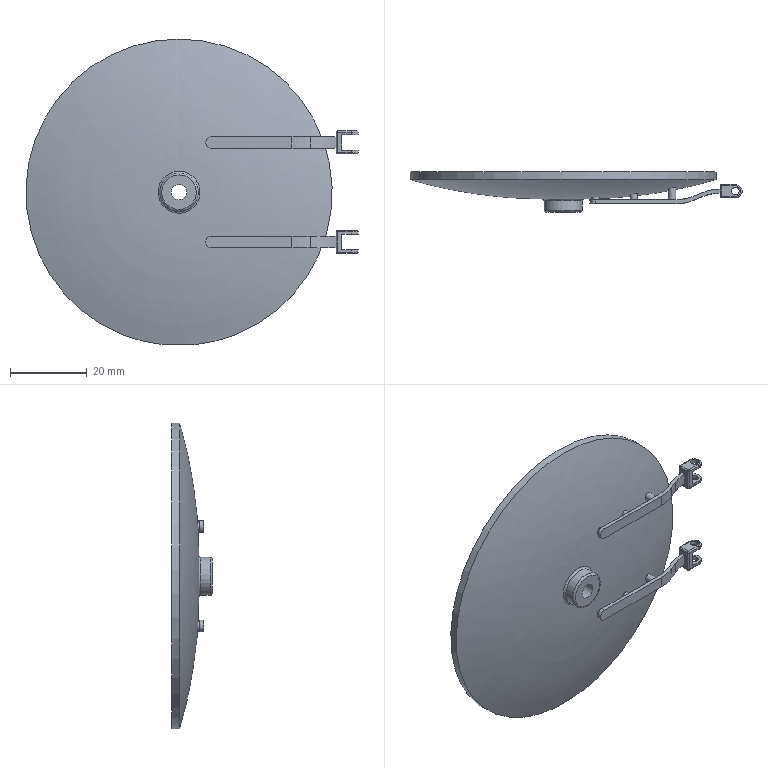Part | STEP file | 1-56.19 | 1 solid | 88 faces | box 86.75 x 10.5 x 80 mm | volume 24295 mm3 | cylinder 43 | plane 30 | sphere 8 | torus 6 | spline 1 | commonest cylinder face diameters 0.707 x16 2 x10 3.5 x4 23 x4 25 x4 3 x2